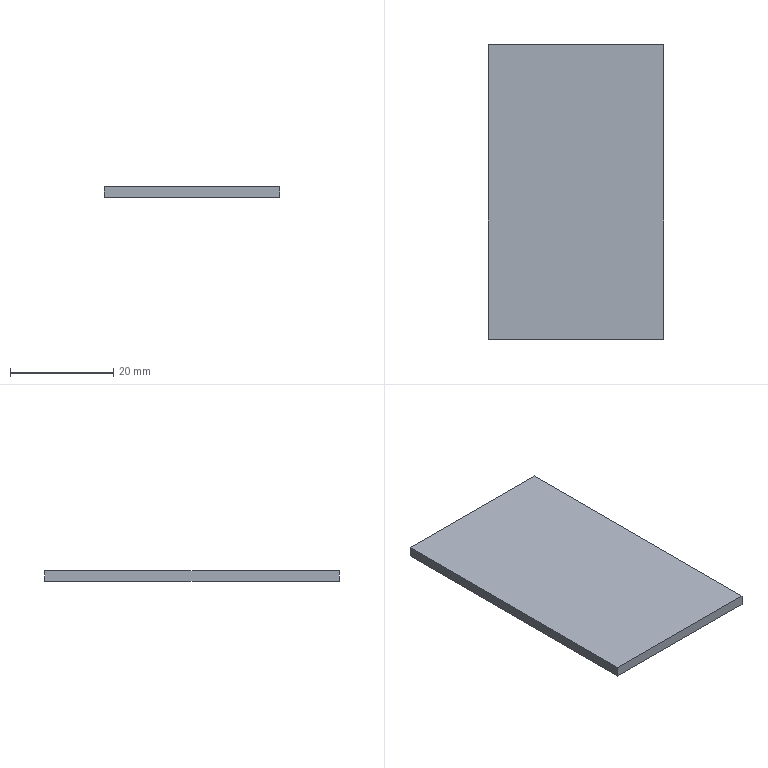Part | STEP file | 03-Sealing plate | 1 solid | 6 faces | box 34 x 57 x 2 mm | volume 3876 mm3 | plane 6
STEP:
#1=CARTESIAN_POINT('',(0.,0.,0.));
#2=DIRECTION('',(0.,0.,1.));
#3=DIRECTION('',(1.,0.,0.));
#4=AXIS2_PLACEMENT_3D('',#1,#2,#3);
#5=CARTESIAN_POINT('',(0.,0.,0.));
#6=VERTEX_POINT('',#5);
#7=CARTESIAN_POINT('',(0.,-57.,0.));
#8=VERTEX_POINT('',#7);
#9=CARTESIAN_POINT('',(0.,0.,0.));
#10=DIRECTION('',(0.,-1.,0.));
#11=VECTOR('',#10,1.);
#12=LINE('',#9,#11);
#13=CARTESIAN_POINT('',(0.,0.,2.));
#14=DIRECTION('',(1.,0.,0.));
#15=DIRECTION('',(0.,1.,0.));
#16=AXIS2_PLACEMENT_3D('',#13,#14,#15);
#17=PLANE('',#16);
#18=CARTESIAN_POINT('',(0.,-2.));
#19=DIRECTION('',(-1.,0.));
#20=VECTOR('',#19,1.);
#21=LINE('',#18,#20);
#22=(GEOMETRIC_REPRESENTATION_CONTEXT(2)PARAMETRIC_REPRESENTATION_CONTEXT()REPRESENTATION_CONTEXT('',''));
#23=DEFINITIONAL_REPRESENTATION('',(#21),#22);
#24=PCURVE('',#17,#23);
#25=CARTESIAN_POINT('',(0.,0.,0.));
#26=DIRECTION('',(0.,0.,1.));
#27=DIRECTION('',(1.,0.,0.));
#28=AXIS2_PLACEMENT_3D('',#25,#26,#27);
#29=PLANE('',#28);
#30=CARTESIAN_POINT('',(0.,0.));
#31=DIRECTION('',(0.,-1.));
#32=VECTOR('',#31,1.);
#33=LINE('',#30,#32);
#34=(GEOMETRIC_REPRESENTATION_CONTEXT(2)PARAMETRIC_REPRESENTATION_CONTEXT()REPRESENTATION_CONTEXT('',''));
#35=DEFINITIONAL_REPRESENTATION('',(#33),#34);
#36=PCURVE('',#29,#35);
#37=SURFACE_CURVE('',#12,(#24,#36),.PCURVE_S1.);
#38=EDGE_CURVE('',#6,#8,#37,.T.);
#39=ORIENTED_EDGE('',*,*,#38,.T.);
#40=CARTESIAN_POINT('',(0.,-57.,2.));
#41=VERTEX_POINT('',#40);
#42=CARTESIAN_POINT('',(0.,-57.,2.));
#43=DIRECTION('',(0.,0.,-1.));
#44=VECTOR('',#43,1.);
#45=LINE('',#42,#44);
#46=CARTESIAN_POINT('',(-57.,0.));
#47=DIRECTION('',(0.,-1.));
#48=VECTOR('',#47,1.);
#49=LINE('',#46,#48);
#50=(GEOMETRIC_REPRESENTATION_CONTEXT(2)PARAMETRIC_REPRESENTATION_CONTEXT()REPRESENTATION_CONTEXT('',''));
#51=DEFINITIONAL_REPRESENTATION('',(#49),#50);
#52=PCURVE('',#17,#51);
#53=CARTESIAN_POINT('',(0.,-57.,2.));
#54=DIRECTION('',(0.,1.,0.));
#55=DIRECTION('',(0.,0.,1.));
#56=AXIS2_PLACEMENT_3D('',#53,#54,#55);
#57=PLANE('',#56);
#58=CARTESIAN_POINT('',(0.,0.));
#59=DIRECTION('',(-1.,0.));
#60=VECTOR('',#59,1.);
#61=LINE('',#58,#60);
#62=(GEOMETRIC_REPRESENTATION_CONTEXT(2)PARAMETRIC_REPRESENTATION_CONTEXT()REPRESENTATION_CONTEXT('',''));
#63=DEFINITIONAL_REPRESENTATION('',(#61),#62);
#64=PCURVE('',#57,#63);
#65=SURFACE_CURVE('',#45,(#52,#64),.PCURVE_S1.);
#66=EDGE_CURVE('',#41,#8,#65,.T.);
#67=ORIENTED_EDGE('',*,*,#66,.F.);
#68=CARTESIAN_POINT('',(0.,0.,2.));
#69=VERTEX_POINT('',#68);
#70=CARTESIAN_POINT('',(0.,0.,2.));
#71=DIRECTION('',(0.,-1.,0.));
#72=VECTOR('',#71,1.);
#73=LINE('',#70,#72);
#74=CARTESIAN_POINT('',(0.,0.));
#75=DIRECTION('',(-1.,0.));
#76=VECTOR('',#75,1.);
#77=LINE('',#74,#76);
#78=(GEOMETRIC_REPRESENTATION_CONTEXT(2)PARAMETRIC_REPRESENTATION_CONTEXT()REPRESENTATION_CONTEXT('',''));
#79=DEFINITIONAL_REPRESENTATION('',(#77),#78);
#80=PCURVE('',#17,#79);
#81=CARTESIAN_POINT('',(0.,0.,2.));
#82=DIRECTION('',(0.,0.,1.));
#83=DIRECTION('',(1.,0.,0.));
#84=AXIS2_PLACEMENT_3D('',#81,#82,#83);
#85=PLANE('',#84);
#86=CARTESIAN_POINT('',(0.,0.));
#87=DIRECTION('',(0.,-1.));
#88=VECTOR('',#87,1.);
#89=LINE('',#86,#88);
#90=(GEOMETRIC_REPRESENTATION_CONTEXT(2)PARAMETRIC_REPRESENTATION_CONTEXT()REPRESENTATION_CONTEXT('',''));
#91=DEFINITIONAL_REPRESENTATION('',(#89),#90);
#92=PCURVE('',#85,#91);
#93=SURFACE_CURVE('',#73,(#80,#92),.PCURVE_S1.);
#94=EDGE_CURVE('',#69,#41,#93,.T.);
#95=ORIENTED_EDGE('',*,*,#94,.F.);
#96=CARTESIAN_POINT('',(0.,0.,2.));
#97=DIRECTION('',(0.,0.,-1.));
#98=VECTOR('',#97,1.);
#99=LINE('',#96,#98);
#100=CARTESIAN_POINT('',(0.,0.));
#101=DIRECTION('',(0.,-1.));
#102=VECTOR('',#101,1.);
#103=LINE('',#100,#102);
#104=(GEOMETRIC_REPRESENTATION_CONTEXT(2)PARAMETRIC_REPRESENTATION_CONTEXT()REPRESENTATION_CONTEXT('',''));
#105=DEFINITIONAL_REPRESENTATION('',(#103),#104);
#106=PCURVE('',#17,#105);
#107=CARTESIAN_POINT('',(0.,0.,2.));
#108=DIRECTION('',(0.,-1.,0.));
#109=DIRECTION('',(0.,0.,-1.));
#110=AXIS2_PLACEMENT_3D('',#107,#108,#109);
#111=PLANE('',#110);
#112=CARTESIAN_POINT('',(0.,0.));
#113=DIRECTION('',(1.,0.));
#114=VECTOR('',#113,1.);
#115=LINE('',#112,#114);
#116=(GEOMETRIC_REPRESENTATION_CONTEXT(2)PARAMETRIC_REPRESENTATION_CONTEXT()REPRESENTATION_CONTEXT('',''));
#117=DEFINITIONAL_REPRESENTATION('',(#115),#116);
#118=PCURVE('',#111,#117);
#119=SURFACE_CURVE('',#99,(#106,#118),.PCURVE_S1.);
#120=EDGE_CURVE('',#69,#6,#119,.T.);
#121=ORIENTED_EDGE('',*,*,#120,.T.);
#122=EDGE_LOOP('',(#39,#67,#95,#121));
#123=FACE_BOUND('',#122,.T.);
#124=ADVANCED_FACE('',(#123),#17,.F.);
#125=CARTESIAN_POINT('',(34.,-57.,0.));
#126=VERTEX_POINT('',#125);
#127=CARTESIAN_POINT('',(0.,-57.,0.));
#128=DIRECTION('',(1.,0.,0.));
#129=VECTOR('',#128,1.);
#130=LINE('',#127,#129);
#131=CARTESIAN_POINT('',(-2.,0.));
#132=DIRECTION('',(0.,1.));
#133=VECTOR('',#132,1.);
#134=LINE('',#131,#133);
#135=(GEOMETRIC_REPRESENTATION_CONTEXT(2)PARAMETRIC_REPRESENTATION_CONTEXT()REPRESENTATION_CONTEXT('',''));
#136=DEFINITIONAL_REPRESENTATION('',(#134),#135);
#137=PCURVE('',#57,#136);
#138=CARTESIAN_POINT('',(0.,-57.));
#139=DIRECTION('',(1.,0.));
#140=VECTOR('',#139,1.);
#141=LINE('',#138,#140);
#142=(GEOMETRIC_REPRESENTATION_CONTEXT(2)PARAMETRIC_REPRESENTATION_CONTEXT()REPRESENTATION_CONTEXT('',''));
#143=DEFINITIONAL_REPRESENTATION('',(#141),#142);
#144=PCURVE('',#29,#143);
#145=SURFACE_CURVE('',#130,(#137,#144),.PCURVE_S1.);
#146=EDGE_CURVE('',#8,#126,#145,.T.);
#147=ORIENTED_EDGE('',*,*,#146,.T.);
#148=CARTESIAN_POINT('',(34.,-57.,2.));
#149=VERTEX_POINT('',#148);
#150=CARTESIAN_POINT('',(34.,-57.,2.));
#151=DIRECTION('',(0.,0.,-1.));
#152=VECTOR('',#151,1.);
#153=LINE('',#150,#152);
#154=CARTESIAN_POINT('',(0.,34.));
#155=DIRECTION('',(-1.,0.));
#156=VECTOR('',#155,1.);
#157=LINE('',#154,#156);
#158=(GEOMETRIC_REPRESENTATION_CONTEXT(2)PARAMETRIC_REPRESENTATION_CONTEXT()REPRESENTATION_CONTEXT('',''));
#159=DEFINITIONAL_REPRESENTATION('',(#157),#158);
#160=PCURVE('',#57,#159);
#161=CARTESIAN_POINT('',(34.,0.,2.));
#162=DIRECTION('',(-1.,0.,0.));
#163=DIRECTION('',(0.,-1.,0.));
#164=AXIS2_PLACEMENT_3D('',#161,#162,#163);
#165=PLANE('',#164);
#166=CARTESIAN_POINT('',(57.,0.));
#167=DIRECTION('',(0.,-1.));
#168=VECTOR('',#167,1.);
#169=LINE('',#166,#168);
#170=(GEOMETRIC_REPRESENTATION_CONTEXT(2)PARAMETRIC_REPRESENTATION_CONTEXT()REPRESENTATION_CONTEXT('',''));
#171=DEFINITIONAL_REPRESENTATION('',(#169),#170);
#172=PCURVE('',#165,#171);
#173=SURFACE_CURVE('',#153,(#160,#172),.PCURVE_S1.);
#174=EDGE_CURVE('',#149,#126,#173,.T.);
#175=ORIENTED_EDGE('',*,*,#174,.F.);
#176=CARTESIAN_POINT('',(0.,-57.,2.));
#177=DIRECTION('',(1.,0.,0.));
#178=VECTOR('',#177,1.);
#179=LINE('',#176,#178);
#180=CARTESIAN_POINT('',(0.,0.));
#181=DIRECTION('',(0.,1.));
#182=VECTOR('',#181,1.);
#183=LINE('',#180,#182);
#184=(GEOMETRIC_REPRESENTATION_CONTEXT(2)PARAMETRIC_REPRESENTATION_CONTEXT()REPRESENTATION_CONTEXT('',''));
#185=DEFINITIONAL_REPRESENTATION('',(#183),#184);
#186=PCURVE('',#57,#185);
#187=CARTESIAN_POINT('',(0.,-57.));
#188=DIRECTION('',(1.,0.));
#189=VECTOR('',#188,1.);
#190=LINE('',#187,#189);
#191=(GEOMETRIC_REPRESENTATION_CONTEXT(2)PARAMETRIC_REPRESENTATION_CONTEXT()REPRESENTATION_CONTEXT('',''));
#192=DEFINITIONAL_REPRESENTATION('',(#190),#191);
#193=PCURVE('',#85,#192);
#194=SURFACE_CURVE('',#179,(#186,#193),.PCURVE_S1.);
#195=EDGE_CURVE('',#41,#149,#194,.T.);
#196=ORIENTED_EDGE('',*,*,#195,.F.);
#197=ORIENTED_EDGE('',*,*,#66,.T.);
#198=EDGE_LOOP('',(#147,#175,#196,#197));
#199=FACE_BOUND('',#198,.T.);
#200=ADVANCED_FACE('',(#199),#57,.F.);
#201=CARTESIAN_POINT('',(34.,0.,0.));
#202=VERTEX_POINT('',#201);
#203=CARTESIAN_POINT('',(34.,0.,0.));
#204=DIRECTION('',(0.,1.,0.));
#205=VECTOR('',#204,1.);
#206=LINE('',#203,#205);
#207=CARTESIAN_POINT('',(0.,-2.));
#208=DIRECTION('',(-1.,0.));
#209=VECTOR('',#208,1.);
#210=LINE('',#207,#209);
#211=(GEOMETRIC_REPRESENTATION_CONTEXT(2)PARAMETRIC_REPRESENTATION_CONTEXT()REPRESENTATION_CONTEXT('',''));
#212=DEFINITIONAL_REPRESENTATION('',(#210),#211);
#213=PCURVE('',#165,#212);
#214=CARTESIAN_POINT('',(34.,0.));
#215=DIRECTION('',(0.,1.));
#216=VECTOR('',#215,1.);
#217=LINE('',#214,#216);
#218=(GEOMETRIC_REPRESENTATION_CONTEXT(2)PARAMETRIC_REPRESENTATION_CONTEXT()REPRESENTATION_CONTEXT('',''));
#219=DEFINITIONAL_REPRESENTATION('',(#217),#218);
#220=PCURVE('',#29,#219);
#221=SURFACE_CURVE('',#206,(#213,#220),.PCURVE_S1.);
#222=EDGE_CURVE('',#126,#202,#221,.T.);
#223=ORIENTED_EDGE('',*,*,#222,.T.);
#224=CARTESIAN_POINT('',(34.,0.,2.));
#225=VERTEX_POINT('',#224);
#226=CARTESIAN_POINT('',(34.,0.,2.));
#227=DIRECTION('',(0.,0.,-1.));
#228=VECTOR('',#227,1.);
#229=LINE('',#226,#228);
#230=CARTESIAN_POINT('',(0.,0.));
#231=DIRECTION('',(0.,-1.));
#232=VECTOR('',#231,1.);
#233=LINE('',#230,#232);
#234=(GEOMETRIC_REPRESENTATION_CONTEXT(2)PARAMETRIC_REPRESENTATION_CONTEXT()REPRESENTATION_CONTEXT('',''));
#235=DEFINITIONAL_REPRESENTATION('',(#233),#234);
#236=PCURVE('',#165,#235);
#237=CARTESIAN_POINT('',(0.,34.));
#238=DIRECTION('',(1.,0.));
#239=VECTOR('',#238,1.);
#240=LINE('',#237,#239);
#241=(GEOMETRIC_REPRESENTATION_CONTEXT(2)PARAMETRIC_REPRESENTATION_CONTEXT()REPRESENTATION_CONTEXT('',''));
#242=DEFINITIONAL_REPRESENTATION('',(#240),#241);
#243=PCURVE('',#111,#242);
#244=SURFACE_CURVE('',#229,(#236,#243),.PCURVE_S1.);
#245=EDGE_CURVE('',#225,#202,#244,.T.);
#246=ORIENTED_EDGE('',*,*,#245,.F.);
#247=CARTESIAN_POINT('',(34.,0.,2.));
#248=DIRECTION('',(0.,1.,0.));
#249=VECTOR('',#248,1.);
#250=LINE('',#247,#249);
#251=CARTESIAN_POINT('',(0.,0.));
#252=DIRECTION('',(-1.,0.));
#253=VECTOR('',#252,1.);
#254=LINE('',#251,#253);
#255=(GEOMETRIC_REPRESENTATION_CONTEXT(2)PARAMETRIC_REPRESENTATION_CONTEXT()REPRESENTATION_CONTEXT('',''));
#256=DEFINITIONAL_REPRESENTATION('',(#254),#255);
#257=PCURVE('',#165,#256);
#258=CARTESIAN_POINT('',(34.,0.));
#259=DIRECTION('',(0.,1.));
#260=VECTOR('',#259,1.);
#261=LINE('',#258,#260);
#262=(GEOMETRIC_REPRESENTATION_CONTEXT(2)PARAMETRIC_REPRESENTATION_CONTEXT()REPRESENTATION_CONTEXT('',''));
#263=DEFINITIONAL_REPRESENTATION('',(#261),#262);
#264=PCURVE('',#85,#263);
#265=SURFACE_CURVE('',#250,(#257,#264),.PCURVE_S1.);
#266=EDGE_CURVE('',#149,#225,#265,.T.);
#267=ORIENTED_EDGE('',*,*,#266,.F.);
#268=ORIENTED_EDGE('',*,*,#174,.T.);
#269=EDGE_LOOP('',(#223,#246,#267,#268));
#270=FACE_BOUND('',#269,.T.);
#271=ADVANCED_FACE('',(#270),#165,.F.);
#272=CARTESIAN_POINT('',(0.,0.,0.));
#273=DIRECTION('',(-1.,0.,0.));
#274=VECTOR('',#273,1.);
#275=LINE('',#272,#274);
#276=CARTESIAN_POINT('',(2.,0.));
#277=DIRECTION('',(0.,-1.));
#278=VECTOR('',#277,1.);
#279=LINE('',#276,#278);
#280=(GEOMETRIC_REPRESENTATION_CONTEXT(2)PARAMETRIC_REPRESENTATION_CONTEXT()REPRESENTATION_CONTEXT('',''));
#281=DEFINITIONAL_REPRESENTATION('',(#279),#280);
#282=PCURVE('',#111,#281);
#283=CARTESIAN_POINT('',(0.,0.));
#284=DIRECTION('',(-1.,0.));
#285=VECTOR('',#284,1.);
#286=LINE('',#283,#285);
#287=(GEOMETRIC_REPRESENTATION_CONTEXT(2)PARAMETRIC_REPRESENTATION_CONTEXT()REPRESENTATION_CONTEXT('',''));
#288=DEFINITIONAL_REPRESENTATION('',(#286),#287);
#289=PCURVE('',#29,#288);
#290=SURFACE_CURVE('',#275,(#282,#289),.PCURVE_S1.);
#291=EDGE_CURVE('',#202,#6,#290,.T.);
#292=ORIENTED_EDGE('',*,*,#291,.T.);
#293=ORIENTED_EDGE('',*,*,#120,.F.);
#294=CARTESIAN_POINT('',(0.,0.,2.));
#295=DIRECTION('',(-1.,0.,0.));
#296=VECTOR('',#295,1.);
#297=LINE('',#294,#296);
#298=CARTESIAN_POINT('',(0.,0.));
#299=DIRECTION('',(0.,-1.));
#300=VECTOR('',#299,1.);
#301=LINE('',#298,#300);
#302=(GEOMETRIC_REPRESENTATION_CONTEXT(2)PARAMETRIC_REPRESENTATION_CONTEXT()REPRESENTATION_CONTEXT('',''));
#303=DEFINITIONAL_REPRESENTATION('',(#301),#302);
#304=PCURVE('',#111,#303);
#305=CARTESIAN_POINT('',(0.,0.));
#306=DIRECTION('',(-1.,0.));
#307=VECTOR('',#306,1.);
#308=LINE('',#305,#307);
#309=(GEOMETRIC_REPRESENTATION_CONTEXT(2)PARAMETRIC_REPRESENTATION_CONTEXT()REPRESENTATION_CONTEXT('',''));
#310=DEFINITIONAL_REPRESENTATION('',(#308),#309);
#311=PCURVE('',#85,#310);
#312=SURFACE_CURVE('',#297,(#304,#311),.PCURVE_S1.);
#313=EDGE_CURVE('',#225,#69,#312,.T.);
#314=ORIENTED_EDGE('',*,*,#313,.F.);
#315=ORIENTED_EDGE('',*,*,#245,.T.);
#316=EDGE_LOOP('',(#292,#293,#314,#315));
#317=FACE_BOUND('',#316,.T.);
#318=ADVANCED_FACE('',(#317),#111,.F.);
#319=ORIENTED_EDGE('',*,*,#94,.T.);
#320=ORIENTED_EDGE('',*,*,#195,.T.);
#321=ORIENTED_EDGE('',*,*,#266,.T.);
#322=ORIENTED_EDGE('',*,*,#313,.T.);
#323=EDGE_LOOP('',(#319,#320,#321,#322));
#324=FACE_BOUND('',#323,.T.);
#325=ADVANCED_FACE('',(#324),#85,.T.);
#326=ORIENTED_EDGE('',*,*,#38,.F.);
#327=ORIENTED_EDGE('',*,*,#291,.F.);
#328=ORIENTED_EDGE('',*,*,#222,.F.);
#329=ORIENTED_EDGE('',*,*,#146,.F.);
#330=EDGE_LOOP('',(#326,#327,#328,#329));
#331=FACE_BOUND('',#330,.T.);
#332=ADVANCED_FACE('',(#331),#29,.F.);
#333=CLOSED_SHELL('',(#124,#200,#271,#318,#325,#332));
#334=MANIFOLD_SOLID_BREP('',#333);
#335=(LENGTH_UNIT()NAMED_UNIT(*)SI_UNIT(.MILLI.,.METRE.));
#336=UNCERTAINTY_MEASURE_WITH_UNIT(LENGTH_MEASURE(0.0000001),#335,'','');
#337=(NAMED_UNIT(*)PLANE_ANGLE_UNIT()SI_UNIT($,.RADIAN.));
#338=(NAMED_UNIT(*)SI_UNIT($,.STERADIAN.)SOLID_ANGLE_UNIT());
#339=(GEOMETRIC_REPRESENTATION_CONTEXT(3)GLOBAL_UNCERTAINTY_ASSIGNED_CONTEXT((#336))GLOBAL_UNIT_ASSIGNED_CONTEXT((#335,#337,#338))REPRESENTATION_CONTEXT('',''));
#340=ADVANCED_BREP_SHAPE_REPRESENTATION('',(#4,#334),#339);